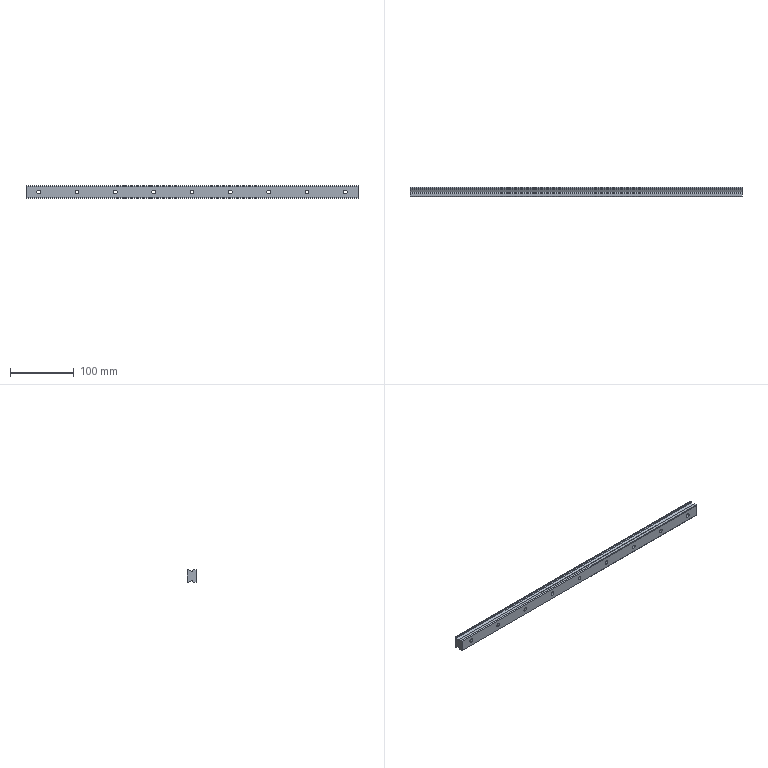Part | STEP file | SSR20XV52020 Track | 1 solid | 74 faces | box 520 x 15.5 x 20 mm | volume 137719 mm3 | cylinder 45 | plane 29 | commonest cylinder face diameters 6 x18 9.5 x18 3.3 x4 2 x3 1.4 x2